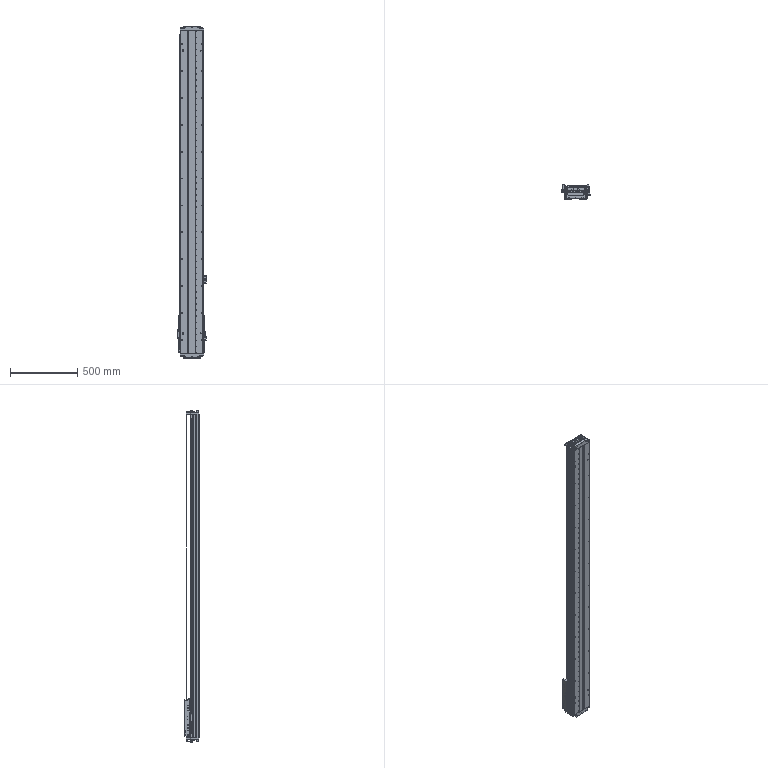Part | SolidWorks | 32 solids | 3119 faces | volume 18345669 mm3 | cylinder 1373 | plane 1355 | cone 249 | spline 142 | commonest cylinder face diameters 4.2 x280 0.6 x161 6.6 x108 4.5 x96 4 x74 3.3 x69